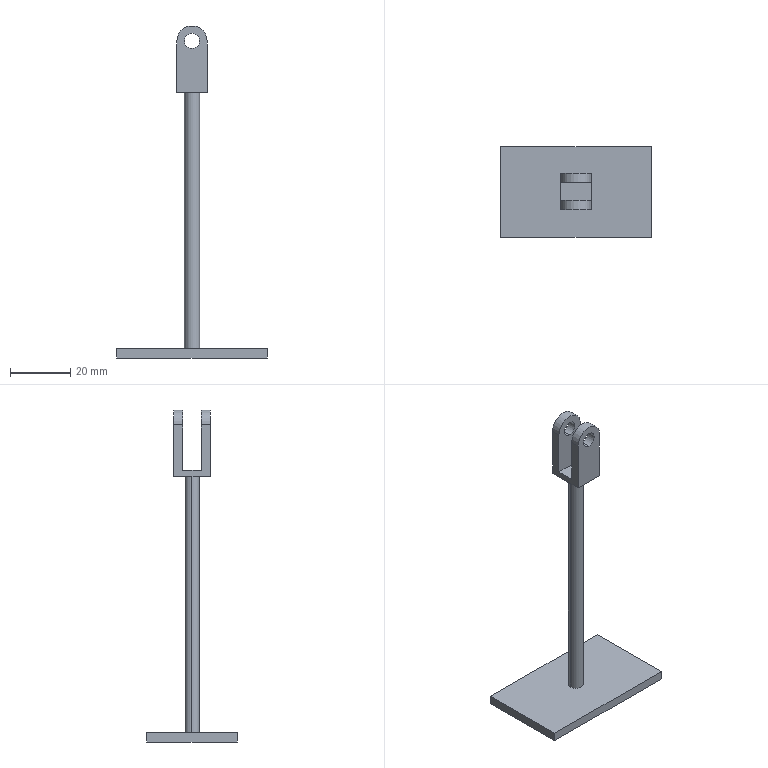Part | SolidWorks | features ICE 4, Extrusion 1 | 1 solid | 22 faces | box 50 x 30 x 110 mm | volume 7427 mm3 | plane 14 | cylinder 8 | commonest cylinder face diameters 5 x6 10 x2
STEP:
#1=CARTESIAN_POINT('',(0.,-3.,107.5));
#2=VERTEX_POINT('',#1);
#3=CARTESIAN_POINT('',(0.,-3.,102.5));
#4=VERTEX_POINT('',#3);
#5=CARTESIAN_POINT('',(0.,-3.,105.));
#6=DIRECTION('',(0.,-1.,0.));
#7=DIRECTION('',(0.,0.,-1.));
#8=AXIS2_PLACEMENT_3D('',#5,#6,#7);
#9=CIRCLE('',#8,2.5);
#10=EDGE_CURVE('',#2,#4,#9,.T.);
#11=ORIENTED_EDGE('',*,*,#10,.F.);
#12=CARTESIAN_POINT('',(0.,-6.,107.5));
#13=VERTEX_POINT('',#12);
#14=CARTESIAN_POINT('',(0.,15.,107.5));
#15=DIRECTION('',(0.,-1.,0.));
#16=VECTOR('',#15,1000.);
#17=LINE('',#14,#16);
#18=EDGE_CURVE('',#2,#13,#17,.T.);
#19=ORIENTED_EDGE('',*,*,#18,.T.);
#20=CARTESIAN_POINT('',(0.,-6.,102.5));
#21=VERTEX_POINT('',#20);
#22=CARTESIAN_POINT('',(0.,-6.,105.));
#23=DIRECTION('',(0.,-1.,0.));
#24=DIRECTION('',(0.,0.,-1.));
#25=AXIS2_PLACEMENT_3D('',#22,#23,#24);
#26=CIRCLE('',#25,2.5);
#27=EDGE_CURVE('',#13,#21,#26,.T.);
#28=ORIENTED_EDGE('',*,*,#27,.T.);
#29=CARTESIAN_POINT('',(0.,15.,102.5));
#30=DIRECTION('',(0.,-1.,0.));
#31=VECTOR('',#30,1000.);
#32=LINE('',#29,#31);
#33=EDGE_CURVE('',#4,#21,#32,.T.);
#34=ORIENTED_EDGE('',*,*,#33,.F.);
#35=EDGE_LOOP('',(#11,#19,#28,#34));
#36=FACE_OUTER_BOUND('',#35,.T.);
#37=CARTESIAN_POINT('',(0.,15.,105.));
#38=DIRECTION('',(0.,-1.,0.));
#39=DIRECTION('',(0.,0.,-1.));
#40=AXIS2_PLACEMENT_3D('',#37,#38,#39);
#41=CYLINDRICAL_SURFACE('',#40,2.5);
#42=ADVANCED_FACE('',(#36),#41,.F.);
#43=CARTESIAN_POINT('',(0.,6.,107.5));
#44=VERTEX_POINT('',#43);
#45=CARTESIAN_POINT('',(0.,6.,102.5));
#46=VERTEX_POINT('',#45);
#47=CARTESIAN_POINT('',(0.,6.,105.));
#48=DIRECTION('',(0.,-1.,0.));
#49=DIRECTION('',(0.,0.,-1.));
#50=AXIS2_PLACEMENT_3D('',#47,#48,#49);
#51=CIRCLE('',#50,2.5);
#52=EDGE_CURVE('',#44,#46,#51,.T.);
#53=ORIENTED_EDGE('',*,*,#52,.F.);
#54=CARTESIAN_POINT('',(0.,3.,107.5));
#55=VERTEX_POINT('',#54);
#56=CARTESIAN_POINT('',(0.,15.,107.5));
#57=DIRECTION('',(0.,-1.,0.));
#58=VECTOR('',#57,1000.);
#59=LINE('',#56,#58);
#60=EDGE_CURVE('',#44,#55,#59,.T.);
#61=ORIENTED_EDGE('',*,*,#60,.T.);
#62=CARTESIAN_POINT('',(0.,3.,102.5));
#63=VERTEX_POINT('',#62);
#64=CARTESIAN_POINT('',(0.,3.,105.));
#65=DIRECTION('',(0.,1.,0.));
#66=DIRECTION('',(0.,0.,1.));
#67=AXIS2_PLACEMENT_3D('',#64,#65,#66);
#68=CIRCLE('',#67,2.5);
#69=EDGE_CURVE('',#63,#55,#68,.T.);
#70=ORIENTED_EDGE('',*,*,#69,.F.);
#71=CARTESIAN_POINT('',(0.,15.,102.5));
#72=DIRECTION('',(0.,-1.,0.));
#73=VECTOR('',#72,1000.);
#74=LINE('',#71,#73);
#75=EDGE_CURVE('',#46,#63,#74,.T.);
#76=ORIENTED_EDGE('',*,*,#75,.F.);
#77=EDGE_LOOP('',(#53,#61,#70,#76));
#78=FACE_OUTER_BOUND('',#77,.T.);
#79=CARTESIAN_POINT('',(0.,15.,105.));
#80=DIRECTION('',(0.,-1.,0.));
#81=DIRECTION('',(0.,0.,-1.));
#82=AXIS2_PLACEMENT_3D('',#79,#80,#81);
#83=CYLINDRICAL_SURFACE('',#82,2.5);
#84=ADVANCED_FACE('',(#78),#83,.F.);
#85=CARTESIAN_POINT('',(2.5,0.,88.));
#86=VERTEX_POINT('',#85);
#87=CARTESIAN_POINT('',(-2.5,0.,88.));
#88=VERTEX_POINT('',#87);
#89=CARTESIAN_POINT('',(0.,0.,88.));
#90=DIRECTION('',(0.,0.,1.));
#91=DIRECTION('',(1.,0.,0.));
#92=AXIS2_PLACEMENT_3D('',#89,#90,#91);
#93=CIRCLE('',#92,2.5);
#94=EDGE_CURVE('',#86,#88,#93,.T.);
#95=ORIENTED_EDGE('',*,*,#94,.F.);
#96=CARTESIAN_POINT('',(2.5,0.,3.));
#97=VERTEX_POINT('',#96);
#98=CARTESIAN_POINT('',(2.5,0.,88.));
#99=DIRECTION('',(0.,0.,-1.));
#100=VECTOR('',#99,1000.);
#101=LINE('',#98,#100);
#102=EDGE_CURVE('',#86,#97,#101,.T.);
#103=ORIENTED_EDGE('',*,*,#102,.T.);
#104=CARTESIAN_POINT('',(-2.5,0.,3.));
#105=VERTEX_POINT('',#104);
#106=CARTESIAN_POINT('',(0.,0.,3.));
#107=DIRECTION('',(0.,0.,1.));
#108=DIRECTION('',(1.,0.,0.));
#109=AXIS2_PLACEMENT_3D('',#106,#107,#108);
#110=CIRCLE('',#109,2.5);
#111=EDGE_CURVE('',#97,#105,#110,.T.);
#112=ORIENTED_EDGE('',*,*,#111,.T.);
#113=CARTESIAN_POINT('',(-2.5,0.,88.));
#114=DIRECTION('',(0.,0.,-1.));
#115=VECTOR('',#114,1000.);
#116=LINE('',#113,#115);
#117=EDGE_CURVE('',#88,#105,#116,.T.);
#118=ORIENTED_EDGE('',*,*,#117,.F.);
#119=EDGE_LOOP('',(#95,#103,#112,#118));
#120=FACE_OUTER_BOUND('',#119,.T.);
#121=CARTESIAN_POINT('',(0.,0.,88.));
#122=DIRECTION('',(0.,0.,-1.));
#123=DIRECTION('',(-1.,0.,0.));
#124=AXIS2_PLACEMENT_3D('',#121,#122,#123);
#125=CYLINDRICAL_SURFACE('',#124,2.5);
#126=ADVANCED_FACE('',(#120),#125,.T.);
#127=CARTESIAN_POINT('',(25.,-15.,0.));
#128=VERTEX_POINT('',#127);
#129=CARTESIAN_POINT('',(25.,15.,0.));
#130=VERTEX_POINT('',#129);
#131=CARTESIAN_POINT('',(25.,15.,0.));
#132=DIRECTION('',(0.,1.,0.));
#133=VECTOR('',#132,1000.);
#134=LINE('',#131,#133);
#135=EDGE_CURVE('',#128,#130,#134,.T.);
#136=ORIENTED_EDGE('',*,*,#135,.T.);
#137=CARTESIAN_POINT('',(25.,15.,3.));
#138=VERTEX_POINT('',#137);
#139=CARTESIAN_POINT('',(25.,15.,3.));
#140=DIRECTION('',(0.,0.,-1.));
#141=VECTOR('',#140,1000.);
#142=LINE('',#139,#141);
#143=EDGE_CURVE('',#138,#130,#142,.T.);
#144=ORIENTED_EDGE('',*,*,#143,.F.);
#145=CARTESIAN_POINT('',(25.,-15.,3.));
#146=VERTEX_POINT('',#145);
#147=CARTESIAN_POINT('',(25.,15.,3.));
#148=DIRECTION('',(0.,1.,0.));
#149=VECTOR('',#148,1000.);
#150=LINE('',#147,#149);
#151=EDGE_CURVE('',#146,#138,#150,.T.);
#152=ORIENTED_EDGE('',*,*,#151,.F.);
#153=CARTESIAN_POINT('',(25.,-15.,3.));
#154=DIRECTION('',(0.,0.,-1.));
#155=VECTOR('',#154,1000.);
#156=LINE('',#153,#155);
#157=EDGE_CURVE('',#146,#128,#156,.T.);
#158=ORIENTED_EDGE('',*,*,#157,.T.);
#159=EDGE_LOOP('',(#136,#144,#152,#158));
#160=FACE_OUTER_BOUND('',#159,.T.);
#161=CARTESIAN_POINT('',(25.,15.,3.));
#162=DIRECTION('',(-1.,0.,0.));
#163=DIRECTION('',(0.,-1.,0.));
#164=AXIS2_PLACEMENT_3D('',#161,#162,#163);
#165=PLANE('',#164);
#166=ADVANCED_FACE('',(#160),#165,.F.);
#167=CARTESIAN_POINT('',(-25.,15.,0.));
#168=VERTEX_POINT('',#167);
#169=CARTESIAN_POINT('',(-25.,15.,0.));
#170=DIRECTION('',(-1.,0.,0.));
#171=VECTOR('',#170,1000.);
#172=LINE('',#169,#171);
#173=EDGE_CURVE('',#130,#168,#172,.T.);
#174=ORIENTED_EDGE('',*,*,#173,.T.);
#175=CARTESIAN_POINT('',(-25.,15.,3.));
#176=VERTEX_POINT('',#175);
#177=CARTESIAN_POINT('',(-25.,15.,3.));
#178=DIRECTION('',(0.,0.,-1.));
#179=VECTOR('',#178,1000.);
#180=LINE('',#177,#179);
#181=EDGE_CURVE('',#176,#168,#180,.T.);
#182=ORIENTED_EDGE('',*,*,#181,.F.);
#183=CARTESIAN_POINT('',(-25.,15.,3.));
#184=DIRECTION('',(-1.,0.,0.));
#185=VECTOR('',#184,1000.);
#186=LINE('',#183,#185);
#187=EDGE_CURVE('',#138,#176,#186,.T.);
#188=ORIENTED_EDGE('',*,*,#187,.F.);
#189=ORIENTED_EDGE('',*,*,#143,.T.);
#190=EDGE_LOOP('',(#174,#182,#188,#189));
#191=FACE_OUTER_BOUND('',#190,.T.);
#192=CARTESIAN_POINT('',(-25.,15.,3.));
#193=DIRECTION('',(0.,-1.,0.));
#194=DIRECTION('',(0.,0.,-1.));
#195=AXIS2_PLACEMENT_3D('',#192,#193,#194);
#196=PLANE('',#195);
#197=ADVANCED_FACE('',(#191),#196,.F.);
#198=CARTESIAN_POINT('',(-25.,-15.,0.));
#199=VERTEX_POINT('',#198);
#200=CARTESIAN_POINT('',(-25.,15.,0.));
#201=DIRECTION('',(0.,-1.,0.));
#202=VECTOR('',#201,1000.);
#203=LINE('',#200,#202);
#204=EDGE_CURVE('',#168,#199,#203,.T.);
#205=ORIENTED_EDGE('',*,*,#204,.T.);
#206=CARTESIAN_POINT('',(-25.,-15.,3.));
#207=VERTEX_POINT('',#206);
#208=CARTESIAN_POINT('',(-25.,-15.,3.));
#209=DIRECTION('',(0.,0.,-1.));
#210=VECTOR('',#209,1000.);
#211=LINE('',#208,#210);
#212=EDGE_CURVE('',#207,#199,#211,.T.);
#213=ORIENTED_EDGE('',*,*,#212,.F.);
#214=CARTESIAN_POINT('',(-25.,15.,3.));
#215=DIRECTION('',(0.,-1.,0.));
#216=VECTOR('',#215,1000.);
#217=LINE('',#214,#216);
#218=EDGE_CURVE('',#176,#207,#217,.T.);
#219=ORIENTED_EDGE('',*,*,#218,.F.);
#220=ORIENTED_EDGE('',*,*,#181,.T.);
#221=EDGE_LOOP('',(#205,#213,#219,#220));
#222=FACE_OUTER_BOUND('',#221,.T.);
#223=CARTESIAN_POINT('',(-25.,15.,3.));
#224=DIRECTION('',(1.,0.,0.));
#225=DIRECTION('',(0.,1.,0.));
#226=AXIS2_PLACEMENT_3D('',#223,#224,#225);
#227=PLANE('',#226);
#228=ADVANCED_FACE('',(#222),#227,.F.);
#229=CARTESIAN_POINT('',(-25.,-15.,0.));
#230=DIRECTION('',(1.,0.,0.));
#231=VECTOR('',#230,1000.);
#232=LINE('',#229,#231);
#233=EDGE_CURVE('',#199,#128,#232,.T.);
#234=ORIENTED_EDGE('',*,*,#233,.T.);
#235=ORIENTED_EDGE('',*,*,#157,.F.);
#236=CARTESIAN_POINT('',(-25.,-15.,3.));
#237=DIRECTION('',(1.,0.,0.));
#238=VECTOR('',#237,1000.);
#239=LINE('',#236,#238);
#240=EDGE_CURVE('',#207,#146,#239,.T.);
#241=ORIENTED_EDGE('',*,*,#240,.F.);
#242=ORIENTED_EDGE('',*,*,#212,.T.);
#243=EDGE_LOOP('',(#234,#235,#241,#242));
#244=FACE_OUTER_BOUND('',#243,.T.);
#245=CARTESIAN_POINT('',(-25.,-15.,3.));
#246=DIRECTION('',(0.,1.,0.));
#247=DIRECTION('',(0.,0.,1.));
#248=AXIS2_PLACEMENT_3D('',#245,#246,#247);
#249=PLANE('',#248);
#250=ADVANCED_FACE('',(#244),#249,.F.);
#251=CARTESIAN_POINT('',(0.,0.,3.));
#252=DIRECTION('',(0.,0.,1.));
#253=DIRECTION('',(1.,0.,0.));
#254=AXIS2_PLACEMENT_3D('',#251,#252,#253);
#255=CIRCLE('',#254,2.5);
#256=EDGE_CURVE('',#105,#97,#255,.T.);
#257=ORIENTED_EDGE('',*,*,#256,.F.);
#258=ORIENTED_EDGE('',*,*,#111,.F.);
#259=EDGE_LOOP('',(#257,#258));
#260=FACE_BOUND('',#259,.T.);
#261=ORIENTED_EDGE('',*,*,#151,.T.);
#262=ORIENTED_EDGE('',*,*,#187,.T.);
#263=ORIENTED_EDGE('',*,*,#218,.T.);
#264=ORIENTED_EDGE('',*,*,#240,.T.);
#265=EDGE_LOOP('',(#261,#262,#263,#264));
#266=FACE_OUTER_BOUND('',#265,.T.);
#267=CARTESIAN_POINT('',(0.,0.,3.));
#268=DIRECTION('',(0.,0.,1.));
#269=DIRECTION('',(1.,0.,0.));
#270=AXIS2_PLACEMENT_3D('',#267,#268,#269);
#271=PLANE('',#270);
#272=ADVANCED_FACE('',(#260,#266),#271,.T.);
#273=ORIENTED_EDGE('',*,*,#135,.F.);
#274=ORIENTED_EDGE('',*,*,#233,.F.);
#275=ORIENTED_EDGE('',*,*,#204,.F.);
#276=ORIENTED_EDGE('',*,*,#173,.F.);
#277=EDGE_LOOP('',(#273,#274,#275,#276));
#278=FACE_OUTER_BOUND('',#277,.T.);
#279=CARTESIAN_POINT('',(0.,0.,0.));
#280=DIRECTION('',(0.,0.,1.));
#281=DIRECTION('',(1.,0.,0.));
#282=AXIS2_PLACEMENT_3D('',#279,#280,#281);
#283=PLANE('',#282);
#284=ADVANCED_FACE('',(#278),#283,.F.);
#285=ORIENTED_EDGE('',*,*,#102,.F.);
#286=CARTESIAN_POINT('',(0.,0.,88.));
#287=DIRECTION('',(0.,0.,1.));
#288=DIRECTION('',(1.,0.,0.));
#289=AXIS2_PLACEMENT_3D('',#286,#287,#288);
#290=CIRCLE('',#289,2.5);
#291=EDGE_CURVE('',#88,#86,#290,.T.);
#292=ORIENTED_EDGE('',*,*,#291,.F.);
#293=ORIENTED_EDGE('',*,*,#117,.T.);
#294=ORIENTED_EDGE('',*,*,#256,.T.);
#295=EDGE_LOOP('',(#285,#292,#293,#294));
#296=FACE_OUTER_BOUND('',#295,.T.);
#297=CARTESIAN_POINT('',(0.,0.,88.));
#298=DIRECTION('',(0.,0.,-1.));
#299=DIRECTION('',(-1.,0.,0.));
#300=AXIS2_PLACEMENT_3D('',#297,#298,#299);
#301=CYLINDRICAL_SURFACE('',#300,2.5);
#302=ADVANCED_FACE('',(#296),#301,.T.);
#303=CARTESIAN_POINT('',(5.,6.,105.));
#304=VERTEX_POINT('',#303);
#305=CARTESIAN_POINT('',(5.,6.,88.));
#306=VERTEX_POINT('',#305);
#307=CARTESIAN_POINT('',(5.,6.,110.));
#308=DIRECTION('',(0.,0.,-1.));
#309=VECTOR('',#308,1000.);
#310=LINE('',#307,#309);
#311=EDGE_CURVE('',#304,#306,#310,.T.);
#312=ORIENTED_EDGE('',*,*,#311,.F.);
#313=CARTESIAN_POINT('',(5.,3.,105.));
#314=VERTEX_POINT('',#313);
#315=CARTESIAN_POINT('',(5.,15.,105.));
#316=DIRECTION('',(0.,-1.,0.));
#317=VECTOR('',#316,1000.);
#318=LINE('',#315,#317);
#319=EDGE_CURVE('',#304,#314,#318,.T.);
#320=ORIENTED_EDGE('',*,*,#319,.T.);
#321=CARTESIAN_POINT('',(5.,3.,90.));
#322=VERTEX_POINT('',#321);
#323=CARTESIAN_POINT('',(5.,3.,110.));
#324=DIRECTION('',(0.,0.,-1.));
#325=VECTOR('',#324,1000.);
#326=LINE('',#323,#325);
#327=EDGE_CURVE('',#314,#322,#326,.T.);
#328=ORIENTED_EDGE('',*,*,#327,.T.);
#329=CARTESIAN_POINT('',(5.,-3.,90.));
#330=VERTEX_POINT('',#329);
#331=CARTESIAN_POINT('',(5.,6.,90.));
#332=DIRECTION('',(0.,1.,0.));
#333=VECTOR('',#332,1000.);
#334=LINE('',#331,#333);
#335=EDGE_CURVE('',#330,#322,#334,.T.);
#336=ORIENTED_EDGE('',*,*,#335,.F.);
#337=CARTESIAN_POINT('',(5.,-3.,105.));
#338=VERTEX_POINT('',#337);
#339=CARTESIAN_POINT('',(5.,-3.,110.));
#340=DIRECTION('',(0.,0.,1.));
#341=VECTOR('',#340,1000.);
#342=LINE('',#339,#341);
#343=EDGE_CURVE('',#330,#338,#342,.T.);
#344=ORIENTED_EDGE('',*,*,#343,.T.);
#345=CARTESIAN_POINT('',(5.,-6.,105.));
#346=VERTEX_POINT('',#345);
#347=CARTESIAN_POINT('',(5.,15.,105.));
#348=DIRECTION('',(0.,-1.,0.));
#349=VECTOR('',#348,1000.);
#350=LINE('',#347,#349);
#351=EDGE_CURVE('',#338,#346,#350,.T.);
#352=ORIENTED_EDGE('',*,*,#351,.T.);
#353=CARTESIAN_POINT('',(5.,-6.,88.));
#354=VERTEX_POINT('',#353);
#355=CARTESIAN_POINT('',(5.,-6.,110.));
#356=DIRECTION('',(0.,0.,-1.));
#357=VECTOR('',#356,1000.);
#358=LINE('',#355,#357);
#359=EDGE_CURVE('',#346,#354,#358,.T.);
#360=ORIENTED_EDGE('',*,*,#359,.T.);
#361=CARTESIAN_POINT('',(5.,6.,88.));
#362=DIRECTION('',(0.,1.,0.));
#363=VECTOR('',#362,1000.);
#364=LINE('',#361,#363);
#365=EDGE_CURVE('',#354,#306,#364,.T.);
#366=ORIENTED_EDGE('',*,*,#365,.T.);
#367=EDGE_LOOP('',(#312,#320,#328,#336,#344,#352,#360,#366));
#368=FACE_OUTER_BOUND('',#367,.T.);
#369=CARTESIAN_POINT('',(5.,6.,110.));
#370=DIRECTION('',(-1.,0.,0.));
#371=DIRECTION('',(0.,-1.,0.));
#372=AXIS2_PLACEMENT_3D('',#369,#370,#371);
#373=PLANE('',#372);
#374=ADVANCED_FACE('',(#368),#373,.F.);
#375=CARTESIAN_POINT('',(0.,6.,105.));
#376=DIRECTION('',(0.,-1.,0.));
#377=DIRECTION('',(0.,0.,-1.));
#378=AXIS2_PLACEMENT_3D('',#375,#376,#377);
#379=CIRCLE('',#378,2.5);
#380=EDGE_CURVE('',#46,#44,#379,.T.);
#381=ORIENTED_EDGE('',*,*,#380,.T.);
#382=ORIENTED_EDGE('',*,*,#52,.T.);
#383=EDGE_LOOP('',(#381,#382));
#384=FACE_BOUND('',#383,.T.);
#385=CARTESIAN_POINT('',(-5.,6.,105.));
#386=VERTEX_POINT('',#385);
#387=CARTESIAN_POINT('',(-5.,6.,88.));
#388=VERTEX_POINT('',#387);
#389=CARTESIAN_POINT('',(-5.,6.,110.));
#390=DIRECTION('',(0.,0.,-1.));
#391=VECTOR('',#390,1000.);
#392=LINE('',#389,#391);
#393=EDGE_CURVE('',#386,#388,#392,.T.);
#394=ORIENTED_EDGE('',*,*,#393,.F.);
#395=CARTESIAN_POINT('',(0.,6.,105.));
#396=DIRECTION('',(0.,1.,0.));
#397=DIRECTION('',(0.,0.,-1.));
#398=AXIS2_PLACEMENT_3D('',#395,#396,#397);
#399=CIRCLE('',#398,5.);
#400=EDGE_CURVE('',#386,#304,#399,.T.);
#401=ORIENTED_EDGE('',*,*,#400,.T.);
#402=ORIENTED_EDGE('',*,*,#311,.T.);
#403=CARTESIAN_POINT('',(-5.,6.,88.));
#404=DIRECTION('',(-1.,0.,0.));
#405=VECTOR('',#404,1000.);
#406=LINE('',#403,#405);
#407=EDGE_CURVE('',#306,#388,#406,.T.);
#408=ORIENTED_EDGE('',*,*,#407,.T.);
#409=EDGE_LOOP('',(#394,#401,#402,#408));
#410=FACE_OUTER_BOUND('',#409,.T.);
#411=CARTESIAN_POINT('',(-5.,6.,110.));
#412=DIRECTION('',(0.,-1.,0.));
#413=DIRECTION('',(0.,0.,-1.));
#414=AXIS2_PLACEMENT_3D('',#411,#412,#413);
#415=PLANE('',#414);
#416=ADVANCED_FACE('',(#384,#410),#415,.F.);
#417=CARTESIAN_POINT('',(-5.,-6.,105.));
#418=VERTEX_POINT('',#417);
#419=CARTESIAN_POINT('',(-5.,-6.,88.));
#420=VERTEX_POINT('',#419);
#421=CARTESIAN_POINT('',(-5.,-6.,110.));
#422=DIRECTION('',(0.,0.,-1.));
#423=VECTOR('',#422,1000.);
#424=LINE('',#421,#423);
#425=EDGE_CURVE('',#418,#420,#424,.T.);
#426=ORIENTED_EDGE('',*,*,#425,.F.);
#427=CARTESIAN_POINT('',(-5.,-3.,105.));
#428=VERTEX_POINT('',#427);
#429=CARTESIAN_POINT('',(-5.,15.,105.));
#430=DIRECTION('',(0.,-1.,0.));
#431=VECTOR('',#430,1000.);
#432=LINE('',#429,#431);
#433=EDGE_CURVE('',#428,#418,#432,.T.);
#434=ORIENTED_EDGE('',*,*,#433,.F.);
#435=CARTESIAN_POINT('',(-5.,-3.,90.));
#436=VERTEX_POINT('',#435);
#437=CARTESIAN_POINT('',(-5.,-3.,110.));
#438=DIRECTION('',(0.,0.,-1.));
#439=VECTOR('',#438,1000.);
#440=LINE('',#437,#439);
#441=EDGE_CURVE('',#428,#436,#440,.T.);
#442=ORIENTED_EDGE('',*,*,#441,.T.);
#443=CARTESIAN_POINT('',(-5.,3.,90.));
#444=VERTEX_POINT('',#443);
#445=CARTESIAN_POINT('',(-5.,6.,90.));
#446=DIRECTION('',(0.,-1.,0.));
#447=VECTOR('',#446,1000.);
#448=LINE('',#445,#447);
#449=EDGE_CURVE('',#444,#436,#448,.T.);
#450=ORIENTED_EDGE('',*,*,#449,.F.);
#451=CARTESIAN_POINT('',(-5.,3.,105.));
#452=VERTEX_POINT('',#451);
#453=CARTESIAN_POINT('',(-5.,3.,110.));
#454=DIRECTION('',(0.,0.,1.));
#455=VECTOR('',#454,1000.);
#456=LINE('',#453,#455);
#457=EDGE_CURVE('',#444,#452,#456,.T.);
#458=ORIENTED_EDGE('',*,*,#457,.T.);
#459=CARTESIAN_POINT('',(-5.,15.,105.));
#460=DIRECTION('',(0.,-1.,0.));
#461=VECTOR('',#460,1000.);
#462=LINE('',#459,#461);
#463=EDGE_CURVE('',#386,#452,#462,.T.);
#464=ORIENTED_EDGE('',*,*,#463,.F.);
#465=ORIENTED_EDGE('',*,*,#393,.T.);
#466=CARTESIAN_POINT('',(-5.,6.,88.));
#467=DIRECTION('',(0.,-1.,0.));
#468=VECTOR('',#467,1000.);
#469=LINE('',#466,#468);
#470=EDGE_CURVE('',#388,#420,#469,.T.);
#471=ORIENTED_EDGE('',*,*,#470,.T.);
#472=EDGE_LOOP('',(#426,#434,#442,#450,#458,#464,#465,#471));
#473=FACE_OUTER_BOUND('',#472,.T.);
#474=CARTESIAN_POINT('',(-5.,6.,110.));
#475=DIRECTION('',(1.,0.,0.));
#476=DIRECTION('',(0.,1.,0.));
#477=AXIS2_PLACEMENT_3D('',#474,#475,#476);
#478=PLANE('',#477);
#479=ADVANCED_FACE('',(#473),#478,.F.);
#480=CARTESIAN_POINT('',(0.,-6.,105.));
#481=DIRECTION('',(0.,-1.,0.));
#482=DIRECTION('',(0.,0.,-1.));
#483=AXIS2_PLACEMENT_3D('',#480,#481,#482);
#484=CIRCLE('',#483,2.5);
#485=EDGE_CURVE('',#21,#13,#484,.T.);
#486=ORIENTED_EDGE('',*,*,#485,.F.);
#487=ORIENTED_EDGE('',*,*,#27,.F.);
#488=EDGE_LOOP('',(#486,#487));
#489=FACE_BOUND('',#488,.T.);
#490=CARTESIAN_POINT('',(0.,-6.,105.));
#491=DIRECTION('',(0.,1.,0.));
#492=DIRECTION('',(0.,0.,-1.));
#493=AXIS2_PLACEMENT_3D('',#490,#491,#492);
#494=CIRCLE('',#493,5.);
#495=EDGE_CURVE('',#418,#346,#494,.T.);
#496=ORIENTED_EDGE('',*,*,#495,.F.);
#497=ORIENTED_EDGE('',*,*,#425,.T.);
#498=CARTESIAN_POINT('',(-5.,-6.,88.));
#499=DIRECTION('',(1.,0.,0.));
#500=VECTOR('',#499,1000.);
#501=LINE('',#498,#500);
#502=EDGE_CURVE('',#420,#354,#501,.T.);
#503=ORIENTED_EDGE('',*,*,#502,.T.);
#504=ORIENTED_EDGE('',*,*,#359,.F.);
#505=EDGE_LOOP('',(#496,#497,#503,#504));
#506=FACE_OUTER_BOUND('',#505,.T.);
#507=CARTESIAN_POINT('',(-5.,-6.,110.));
#508=DIRECTION('',(0.,1.,0.));
#509=DIRECTION('',(0.,0.,1.));
#510=AXIS2_PLACEMENT_3D('',#507,#508,#509);
#511=PLANE('',#510);
#512=ADVANCED_FACE('',(#489,#506),#511,.F.);
#513=ORIENTED_EDGE('',*,*,#291,.T.);
#514=ORIENTED_EDGE('',*,*,#94,.T.);
#515=EDGE_LOOP('',(#513,#514));
#516=FACE_BOUND('',#515,.T.);
#517=ORIENTED_EDGE('',*,*,#365,.F.);
#518=ORIENTED_EDGE('',*,*,#502,.F.);
#519=ORIENTED_EDGE('',*,*,#470,.F.);
#520=ORIENTED_EDGE('',*,*,#407,.F.);
#521=EDGE_LOOP('',(#517,#518,#519,#520));
#522=FACE_OUTER_BOUND('',#521,.T.);
#523=CARTESIAN_POINT('',(0.,0.,88.));
#524=DIRECTION('',(0.,0.,1.));
#525=DIRECTION('',(1.,0.,0.));
#526=AXIS2_PLACEMENT_3D('',#523,#524,#525);
#527=PLANE('',#526);
#528=ADVANCED_FACE('',(#516,#522),#527,.F.);
#529=ORIENTED_EDGE('',*,*,#335,.T.);
#530=CARTESIAN_POINT('',(-8.798,3.,90.));
#531=DIRECTION('',(-1.,0.,0.));
#532=VECTOR('',#531,1000.);
#533=LINE('',#530,#532);
#534=EDGE_CURVE('',#322,#444,#533,.T.);
#535=ORIENTED_EDGE('',*,*,#534,.T.);
#536=ORIENTED_EDGE('',*,*,#449,.T.);
#537=CARTESIAN_POINT('',(-8.798,-3.,90.));
#538=DIRECTION('',(1.,0.,0.));
#539=VECTOR('',#538,1000.);
#540=LINE('',#537,#539);
#541=EDGE_CURVE('',#436,#330,#540,.T.);
#542=ORIENTED_EDGE('',*,*,#541,.T.);
#543=EDGE_LOOP('',(#529,#535,#536,#542));
#544=FACE_OUTER_BOUND('',#543,.T.);
#545=CARTESIAN_POINT('',(0.,0.,90.));
#546=DIRECTION('',(0.,0.,1.));
#547=DIRECTION('',(1.,0.,0.));
#548=AXIS2_PLACEMENT_3D('',#545,#546,#547);
#549=PLANE('',#548);
#550=ADVANCED_FACE('',(#544),#549,.T.);
#551=CARTESIAN_POINT('',(0.,-3.,105.));
#552=DIRECTION('',(0.,-1.,0.));
#553=DIRECTION('',(0.,0.,-1.));
#554=AXIS2_PLACEMENT_3D('',#551,#552,#553);
#555=CIRCLE('',#554,2.5);
#556=EDGE_CURVE('',#4,#2,#555,.T.);
#557=ORIENTED_EDGE('',*,*,#556,.T.);
#558=ORIENTED_EDGE('',*,*,#10,.T.);
#559=EDGE_LOOP('',(#557,#558));
#560=FACE_BOUND('',#559,.T.);
#561=ORIENTED_EDGE('',*,*,#441,.F.);
#562=CARTESIAN_POINT('',(0.,-3.,105.));
#563=DIRECTION('',(0.,1.,0.));
#564=DIRECTION('',(0.,0.,-1.));
#565=AXIS2_PLACEMENT_3D('',#562,#563,#564);
#566=CIRCLE('',#565,5.);
#567=EDGE_CURVE('',#428,#338,#566,.T.);
#568=ORIENTED_EDGE('',*,*,#567,.T.);
#569=ORIENTED_EDGE('',*,*,#343,.F.);
#570=ORIENTED_EDGE('',*,*,#541,.F.);
#571=EDGE_LOOP('',(#561,#568,#569,#570));
#572=FACE_OUTER_BOUND('',#571,.T.);
#573=CARTESIAN_POINT('',(-8.798,-3.,90.));
#574=DIRECTION('',(0.,-1.,0.));
#575=DIRECTION('',(0.,0.,-1.));
#576=AXIS2_PLACEMENT_3D('',#573,#574,#575);
#577=PLANE('',#576);
#578=ADVANCED_FACE('',(#560,#572),#577,.F.);
#579=ORIENTED_EDGE('',*,*,#69,.T.);
#580=CARTESIAN_POINT('',(0.,3.,105.));
#581=DIRECTION('',(0.,1.,0.));
#582=DIRECTION('',(0.,0.,1.));
#583=AXIS2_PLACEMENT_3D('',#580,#581,#582);
#584=CIRCLE('',#583,2.5);
#585=EDGE_CURVE('',#55,#63,#584,.T.);
#586=ORIENTED_EDGE('',*,*,#585,.T.);
#587=EDGE_LOOP('',(#579,#586));
#588=FACE_BOUND('',#587,.T.);
#589=CARTESIAN_POINT('',(0.,3.,105.));
#590=DIRECTION('',(0.,-1.,0.));
#591=DIRECTION('',(0.,0.,1.));
#592=AXIS2_PLACEMENT_3D('',#589,#590,#591);
#593=CIRCLE('',#592,5.);
#594=EDGE_CURVE('',#314,#452,#593,.T.);
#595=ORIENTED_EDGE('',*,*,#594,.T.);
#596=ORIENTED_EDGE('',*,*,#457,.F.);
#597=ORIENTED_EDGE('',*,*,#534,.F.);
#598=ORIENTED_EDGE('',*,*,#327,.F.);
#599=EDGE_LOOP('',(#595,#596,#597,#598));
#600=FACE_OUTER_BOUND('',#599,.T.);
#601=CARTESIAN_POINT('',(-8.798,3.,90.));
#602=DIRECTION('',(0.,1.,0.));
#603=DIRECTION('',(0.,0.,1.));
#604=AXIS2_PLACEMENT_3D('',#601,#602,#603);
#605=PLANE('',#604);
#606=ADVANCED_FACE('',(#588,#600),#605,.F.);
#607=ORIENTED_EDGE('',*,*,#60,.F.);
#608=ORIENTED_EDGE('',*,*,#380,.F.);
#609=ORIENTED_EDGE('',*,*,#75,.T.);
#610=ORIENTED_EDGE('',*,*,#585,.F.);
#611=EDGE_LOOP('',(#607,#608,#609,#610));
#612=FACE_OUTER_BOUND('',#611,.T.);
#613=CARTESIAN_POINT('',(0.,15.,105.));
#614=DIRECTION('',(0.,-1.,0.));
#615=DIRECTION('',(0.,0.,-1.));
#616=AXIS2_PLACEMENT_3D('',#613,#614,#615);
#617=CYLINDRICAL_SURFACE('',#616,2.5);
#618=ADVANCED_FACE('',(#612),#617,.F.);
#619=ORIENTED_EDGE('',*,*,#463,.T.);
#620=ORIENTED_EDGE('',*,*,#594,.F.);
#621=ORIENTED_EDGE('',*,*,#319,.F.);
#622=ORIENTED_EDGE('',*,*,#400,.F.);
#623=EDGE_LOOP('',(#619,#620,#621,#622));
#624=FACE_OUTER_BOUND('',#623,.T.);
#625=CARTESIAN_POINT('',(0.,15.,105.));
#626=DIRECTION('',(0.,-1.,0.));
#627=DIRECTION('',(0.,0.,-1.));
#628=AXIS2_PLACEMENT_3D('',#625,#626,#627);
#629=CYLINDRICAL_SURFACE('',#628,5.);
#630=ADVANCED_FACE('',(#624),#629,.T.);
#631=ORIENTED_EDGE('',*,*,#18,.F.);
#632=ORIENTED_EDGE('',*,*,#556,.F.);
#633=ORIENTED_EDGE('',*,*,#33,.T.);
#634=ORIENTED_EDGE('',*,*,#485,.T.);
#635=EDGE_LOOP('',(#631,#632,#633,#634));
#636=FACE_OUTER_BOUND('',#635,.T.);
#637=CARTESIAN_POINT('',(0.,15.,105.));
#638=DIRECTION('',(0.,-1.,0.));
#639=DIRECTION('',(0.,0.,-1.));
#640=AXIS2_PLACEMENT_3D('',#637,#638,#639);
#641=CYLINDRICAL_SURFACE('',#640,2.5);
#642=ADVANCED_FACE('',(#636),#641,.F.);
#643=ORIENTED_EDGE('',*,*,#495,.T.);
#644=ORIENTED_EDGE('',*,*,#351,.F.);
#645=ORIENTED_EDGE('',*,*,#567,.F.);
#646=ORIENTED_EDGE('',*,*,#433,.T.);
#647=EDGE_LOOP('',(#643,#644,#645,#646));
#648=FACE_OUTER_BOUND('',#647,.T.);
#649=CARTESIAN_POINT('',(0.,15.,105.));
#650=DIRECTION('',(0.,-1.,0.));
#651=DIRECTION('',(0.,0.,-1.));
#652=AXIS2_PLACEMENT_3D('',#649,#650,#651);
#653=CYLINDRICAL_SURFACE('',#652,5.);
#654=ADVANCED_FACE('',(#648),#653,.T.);
#655=CLOSED_SHELL('',(#42,#84,#126,#166,#197,#228,#250,#272,#284,#302,#374,#416,#479,#512,#528,#550,#578,#606,#618,#630,#642,#654));
#656=MANIFOLD_SOLID_BREP('',#655);
#657=CARTESIAN_POINT('',(0.,0.,0.));
#658=DIRECTION('',(0.,0.,1.));
#659=DIRECTION('',(1.,0.,0.));
#660=AXIS2_PLACEMENT_3D('',#657,#658,#659);
#661=(LENGTH_UNIT()NAMED_UNIT(*)SI_UNIT(.MILLI.,.METRE.));
#662=UNCERTAINTY_MEASURE_WITH_UNIT(LENGTH_MEASURE(0.00001),#661,'','');
#663=(NAMED_UNIT(*)PLANE_ANGLE_UNIT()SI_UNIT($,.RADIAN.));
#664=(NAMED_UNIT(*)SI_UNIT($,.STERADIAN.)SOLID_ANGLE_UNIT());
#665=(GEOMETRIC_REPRESENTATION_CONTEXT(3)GLOBAL_UNCERTAINTY_ASSIGNED_CONTEXT((#662))GLOBAL_UNIT_ASSIGNED_CONTEXT((#661,#663,#664))REPRESENTATION_CONTEXT('',''));
#666=ADVANCED_BREP_SHAPE_REPRESENTATION('',(#656,#660),#665);